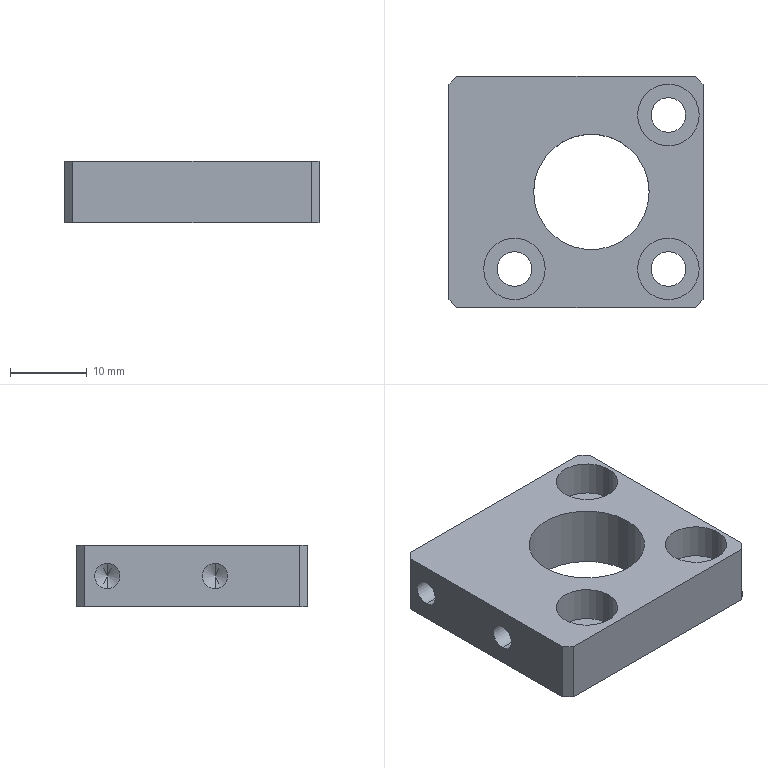Part | STEP file | FBDS-CS-015 | 1 solid | 35 faces | box 33 x 30 x 8 mm | volume 5456 mm3 | cylinder 18 | plane 13 | cone 4 | commonest cylinder face diameters 4.5 x6 8 x6 3.3 x4 15 x2
STEP:
#1=CARTESIAN_POINT('',(-8.4,11.,2.35));
#2=VERTEX_POINT('',#1);
#3=CARTESIAN_POINT('',(-8.4,11.,5.65));
#4=VERTEX_POINT('',#3);
#5=CARTESIAN_POINT('',(-8.4,11.,4.));
#6=DIRECTION('',(-1.,0.,0.));
#7=DIRECTION('',(0.,0.,1.));
#8=AXIS2_PLACEMENT_3D('',#5,#6,#7);
#9=CIRCLE('',#8,1.65);
#10=EDGE_CURVE('',#2,#4,#9,.T.);
#11=ORIENTED_EDGE('',*,*,#10,.F.);
#12=CARTESIAN_POINT('',(-18.5,11.,2.35));
#13=VERTEX_POINT('',#12);
#14=CARTESIAN_POINT('',(-18.5,11.,2.35));
#15=DIRECTION('',(-1.,0.,0.));
#16=VECTOR('',#15,1000.);
#17=LINE('',#14,#16);
#18=EDGE_CURVE('',#2,#13,#17,.T.);
#19=ORIENTED_EDGE('',*,*,#18,.T.);
#20=CARTESIAN_POINT('',(-18.5,11.,5.65));
#21=VERTEX_POINT('',#20);
#22=CARTESIAN_POINT('',(-18.5,11.,4.));
#23=DIRECTION('',(-1.,0.,0.));
#24=DIRECTION('',(0.,0.,1.));
#25=AXIS2_PLACEMENT_3D('',#22,#23,#24);
#26=CIRCLE('',#25,1.65);
#27=EDGE_CURVE('',#13,#21,#26,.T.);
#28=ORIENTED_EDGE('',*,*,#27,.T.);
#29=CARTESIAN_POINT('',(-18.5,11.,5.65));
#30=DIRECTION('',(-1.,0.,0.));
#31=VECTOR('',#30,1000.);
#32=LINE('',#29,#31);
#33=EDGE_CURVE('',#4,#21,#32,.T.);
#34=ORIENTED_EDGE('',*,*,#33,.F.);
#35=EDGE_LOOP('',(#11,#19,#28,#34));
#36=FACE_OUTER_BOUND('',#35,.T.);
#37=CARTESIAN_POINT('',(-18.5,11.,4.));
#38=DIRECTION('',(-1.,0.,0.));
#39=DIRECTION('',(0.,0.,1.));
#40=AXIS2_PLACEMENT_3D('',#37,#38,#39);
#41=CYLINDRICAL_SURFACE('',#40,1.65);
#42=ADVANCED_FACE('',(#36),#41,.F.);
#43=CARTESIAN_POINT('',(-7.409,11.,4.));
#44=VERTEX_POINT('',#43);
#45=CARTESIAN_POINT('',(-8.4,11.,5.65));
#46=DIRECTION('',(-0.515,0.,0.8572));
#47=VECTOR('',#46,1000.);
#48=LINE('',#45,#47);
#49=EDGE_CURVE('',#44,#4,#48,.T.);
#50=ORIENTED_EDGE('',*,*,#49,.F.);
#51=CARTESIAN_POINT('',(-8.4,11.,2.35));
#52=DIRECTION('',(-0.515,0.,-0.8572));
#53=VECTOR('',#52,1000.);
#54=LINE('',#51,#53);
#55=EDGE_CURVE('',#44,#2,#54,.T.);
#56=ORIENTED_EDGE('',*,*,#55,.T.);
#57=ORIENTED_EDGE('',*,*,#10,.T.);
#58=EDGE_LOOP('',(#50,#56,#57));
#59=FACE_OUTER_BOUND('',#58,.T.);
#60=CARTESIAN_POINT('',(-8.4,11.,4.));
#61=DIRECTION('',(-1.,0.,0.));
#62=DIRECTION('',(0.,0.,1.));
#63=AXIS2_PLACEMENT_3D('',#60,#61,#62);
#64=CONICAL_SURFACE('',#63,1.65,1.03);
#65=ADVANCED_FACE('',(#59),#64,.F.);
#66=CARTESIAN_POINT('',(-8.4,-3.,2.35));
#67=VERTEX_POINT('',#66);
#68=CARTESIAN_POINT('',(-8.4,-3.,5.65));
#69=VERTEX_POINT('',#68);
#70=CARTESIAN_POINT('',(-8.4,-3.,4.));
#71=DIRECTION('',(-1.,0.,0.));
#72=DIRECTION('',(0.,0.,1.));
#73=AXIS2_PLACEMENT_3D('',#70,#71,#72);
#74=CIRCLE('',#73,1.65);
#75=EDGE_CURVE('',#67,#69,#74,.T.);
#76=ORIENTED_EDGE('',*,*,#75,.F.);
#77=CARTESIAN_POINT('',(-18.5,-3.,2.35));
#78=VERTEX_POINT('',#77);
#79=CARTESIAN_POINT('',(-18.5,-3.,2.35));
#80=DIRECTION('',(-1.,0.,0.));
#81=VECTOR('',#80,1000.);
#82=LINE('',#79,#81);
#83=EDGE_CURVE('',#67,#78,#82,.T.);
#84=ORIENTED_EDGE('',*,*,#83,.T.);
#85=CARTESIAN_POINT('',(-18.5,-3.,5.65));
#86=VERTEX_POINT('',#85);
#87=CARTESIAN_POINT('',(-18.5,-3.,4.));
#88=DIRECTION('',(-1.,0.,0.));
#89=DIRECTION('',(0.,0.,1.));
#90=AXIS2_PLACEMENT_3D('',#87,#88,#89);
#91=CIRCLE('',#90,1.65);
#92=EDGE_CURVE('',#78,#86,#91,.T.);
#93=ORIENTED_EDGE('',*,*,#92,.T.);
#94=CARTESIAN_POINT('',(-18.5,-3.,5.65));
#95=DIRECTION('',(-1.,0.,0.));
#96=VECTOR('',#95,1000.);
#97=LINE('',#94,#96);
#98=EDGE_CURVE('',#69,#86,#97,.T.);
#99=ORIENTED_EDGE('',*,*,#98,.F.);
#100=EDGE_LOOP('',(#76,#84,#93,#99));
#101=FACE_OUTER_BOUND('',#100,.T.);
#102=CARTESIAN_POINT('',(-18.5,-3.,4.));
#103=DIRECTION('',(-1.,0.,0.));
#104=DIRECTION('',(0.,0.,1.));
#105=AXIS2_PLACEMENT_3D('',#102,#103,#104);
#106=CYLINDRICAL_SURFACE('',#105,1.65);
#107=ADVANCED_FACE('',(#101),#106,.F.);
#108=CARTESIAN_POINT('',(-7.409,-3.,4.));
#109=VERTEX_POINT('',#108);
#110=CARTESIAN_POINT('',(-8.4,-3.,5.65));
#111=DIRECTION('',(-0.515,0.,0.8572));
#112=VECTOR('',#111,1000.);
#113=LINE('',#110,#112);
#114=EDGE_CURVE('',#109,#69,#113,.T.);
#115=ORIENTED_EDGE('',*,*,#114,.F.);
#116=CARTESIAN_POINT('',(-8.4,-3.,2.35));
#117=DIRECTION('',(-0.515,0.,-0.8572));
#118=VECTOR('',#117,1000.);
#119=LINE('',#116,#118);
#120=EDGE_CURVE('',#109,#67,#119,.T.);
#121=ORIENTED_EDGE('',*,*,#120,.T.);
#122=ORIENTED_EDGE('',*,*,#75,.T.);
#123=EDGE_LOOP('',(#115,#121,#122));
#124=FACE_OUTER_BOUND('',#123,.T.);
#125=CARTESIAN_POINT('',(-8.4,-3.,4.));
#126=DIRECTION('',(-1.,0.,0.));
#127=DIRECTION('',(0.,0.,1.));
#128=AXIS2_PLACEMENT_3D('',#125,#126,#127);
#129=CONICAL_SURFACE('',#128,1.65,1.03);
#130=ADVANCED_FACE('',(#124),#129,.F.);
#131=CARTESIAN_POINT('',(-14.,-10.,3.4));
#132=VERTEX_POINT('',#131);
#133=CARTESIAN_POINT('',(-6.,-10.,3.4));
#134=VERTEX_POINT('',#133);
#135=CARTESIAN_POINT('',(-10.,-10.,3.4));
#136=DIRECTION('',(0.,0.,1.));
#137=DIRECTION('',(1.,0.,0.));
#138=AXIS2_PLACEMENT_3D('',#135,#136,#137);
#139=CIRCLE('',#138,4.);
#140=EDGE_CURVE('',#132,#134,#139,.T.);
#141=ORIENTED_EDGE('',*,*,#140,.F.);
#142=CARTESIAN_POINT('',(-14.,-10.,8.));
#143=VERTEX_POINT('',#142);
#144=CARTESIAN_POINT('',(-14.,-10.,8.));
#145=DIRECTION('',(0.,0.,1.));
#146=VECTOR('',#145,1000.);
#147=LINE('',#144,#146);
#148=EDGE_CURVE('',#132,#143,#147,.T.);
#149=ORIENTED_EDGE('',*,*,#148,.T.);
#150=CARTESIAN_POINT('',(-6.,-10.,8.));
#151=VERTEX_POINT('',#150);
#152=CARTESIAN_POINT('',(-10.,-10.,8.));
#153=DIRECTION('',(0.,0.,1.));
#154=DIRECTION('',(1.,0.,0.));
#155=AXIS2_PLACEMENT_3D('',#152,#153,#154);
#156=CIRCLE('',#155,4.);
#157=EDGE_CURVE('',#143,#151,#156,.T.);
#158=ORIENTED_EDGE('',*,*,#157,.T.);
#159=CARTESIAN_POINT('',(-6.,-10.,8.));
#160=DIRECTION('',(0.,0.,1.));
#161=VECTOR('',#160,1000.);
#162=LINE('',#159,#161);
#163=EDGE_CURVE('',#134,#151,#162,.T.);
#164=ORIENTED_EDGE('',*,*,#163,.F.);
#165=EDGE_LOOP('',(#141,#149,#158,#164));
#166=FACE_OUTER_BOUND('',#165,.T.);
#167=CARTESIAN_POINT('',(-10.,-10.,8.));
#168=DIRECTION('',(0.,0.,1.));
#169=DIRECTION('',(1.,0.,0.));
#170=AXIS2_PLACEMENT_3D('',#167,#168,#169);
#171=CYLINDRICAL_SURFACE('',#170,4.);
#172=ADVANCED_FACE('',(#166),#171,.F.);
#173=CARTESIAN_POINT('',(-12.25,-10.,0.));
#174=VERTEX_POINT('',#173);
#175=CARTESIAN_POINT('',(-7.75,-10.,0.));
#176=VERTEX_POINT('',#175);
#177=CARTESIAN_POINT('',(-10.,-10.,0.));
#178=DIRECTION('',(0.,0.,1.));
#179=DIRECTION('',(1.,0.,0.));
#180=AXIS2_PLACEMENT_3D('',#177,#178,#179);
#181=CIRCLE('',#180,2.25);
#182=EDGE_CURVE('',#174,#176,#181,.T.);
#183=ORIENTED_EDGE('',*,*,#182,.F.);
#184=CARTESIAN_POINT('',(-12.25,-10.,3.4));
#185=VERTEX_POINT('',#184);
#186=CARTESIAN_POINT('',(-12.25,-10.,8.));
#187=DIRECTION('',(0.,0.,1.));
#188=VECTOR('',#187,1000.);
#189=LINE('',#186,#188);
#190=EDGE_CURVE('',#174,#185,#189,.T.);
#191=ORIENTED_EDGE('',*,*,#190,.T.);
#192=CARTESIAN_POINT('',(-7.75,-10.,3.4));
#193=VERTEX_POINT('',#192);
#194=CARTESIAN_POINT('',(-10.,-10.,3.4));
#195=DIRECTION('',(0.,0.,1.));
#196=DIRECTION('',(1.,0.,0.));
#197=AXIS2_PLACEMENT_3D('',#194,#195,#196);
#198=CIRCLE('',#197,2.25);
#199=EDGE_CURVE('',#185,#193,#198,.T.);
#200=ORIENTED_EDGE('',*,*,#199,.T.);
#201=CARTESIAN_POINT('',(-7.75,-10.,8.));
#202=DIRECTION('',(0.,0.,1.));
#203=VECTOR('',#202,1000.);
#204=LINE('',#201,#203);
#205=EDGE_CURVE('',#176,#193,#204,.T.);
#206=ORIENTED_EDGE('',*,*,#205,.F.);
#207=EDGE_LOOP('',(#183,#191,#200,#206));
#208=FACE_OUTER_BOUND('',#207,.T.);
#209=CARTESIAN_POINT('',(-10.,-10.,8.));
#210=DIRECTION('',(0.,0.,1.));
#211=DIRECTION('',(1.,0.,0.));
#212=AXIS2_PLACEMENT_3D('',#209,#210,#211);
#213=CYLINDRICAL_SURFACE('',#212,2.25);
#214=ADVANCED_FACE('',(#208),#213,.F.);
#215=CARTESIAN_POINT('',(6.,10.,3.4));
#216=VERTEX_POINT('',#215);
#217=CARTESIAN_POINT('',(14.,10.,3.4));
#218=VERTEX_POINT('',#217);
#219=CARTESIAN_POINT('',(10.,10.,3.4));
#220=DIRECTION('',(0.,0.,1.));
#221=DIRECTION('',(1.,0.,0.));
#222=AXIS2_PLACEMENT_3D('',#219,#220,#221);
#223=CIRCLE('',#222,4.);
#224=EDGE_CURVE('',#216,#218,#223,.T.);
#225=ORIENTED_EDGE('',*,*,#224,.F.);
#226=CARTESIAN_POINT('',(6.,10.,8.));
#227=VERTEX_POINT('',#226);
#228=CARTESIAN_POINT('',(6.,10.,8.));
#229=DIRECTION('',(0.,0.,1.));
#230=VECTOR('',#229,1000.);
#231=LINE('',#228,#230);
#232=EDGE_CURVE('',#216,#227,#231,.T.);
#233=ORIENTED_EDGE('',*,*,#232,.T.);
#234=CARTESIAN_POINT('',(14.,10.,8.));
#235=VERTEX_POINT('',#234);
#236=CARTESIAN_POINT('',(10.,10.,8.));
#237=DIRECTION('',(0.,0.,1.));
#238=DIRECTION('',(1.,0.,0.));
#239=AXIS2_PLACEMENT_3D('',#236,#237,#238);
#240=CIRCLE('',#239,4.);
#241=EDGE_CURVE('',#227,#235,#240,.T.);
#242=ORIENTED_EDGE('',*,*,#241,.T.);
#243=CARTESIAN_POINT('',(14.,10.,8.));
#244=DIRECTION('',(0.,0.,1.));
#245=VECTOR('',#244,1000.);
#246=LINE('',#243,#245);
#247=EDGE_CURVE('',#218,#235,#246,.T.);
#248=ORIENTED_EDGE('',*,*,#247,.F.);
#249=EDGE_LOOP('',(#225,#233,#242,#248));
#250=FACE_OUTER_BOUND('',#249,.T.);
#251=CARTESIAN_POINT('',(10.,10.,8.));
#252=DIRECTION('',(0.,0.,1.));
#253=DIRECTION('',(1.,0.,0.));
#254=AXIS2_PLACEMENT_3D('',#251,#252,#253);
#255=CYLINDRICAL_SURFACE('',#254,4.);
#256=ADVANCED_FACE('',(#250),#255,.F.);
#257=CARTESIAN_POINT('',(7.75,10.,0.));
#258=VERTEX_POINT('',#257);
#259=CARTESIAN_POINT('',(12.25,10.,0.));
#260=VERTEX_POINT('',#259);
#261=CARTESIAN_POINT('',(10.,10.,0.));
#262=DIRECTION('',(0.,0.,1.));
#263=DIRECTION('',(1.,0.,0.));
#264=AXIS2_PLACEMENT_3D('',#261,#262,#263);
#265=CIRCLE('',#264,2.25);
#266=EDGE_CURVE('',#258,#260,#265,.T.);
#267=ORIENTED_EDGE('',*,*,#266,.F.);
#268=CARTESIAN_POINT('',(7.75,10.,3.4));
#269=VERTEX_POINT('',#268);
#270=CARTESIAN_POINT('',(7.75,10.,8.));
#271=DIRECTION('',(0.,0.,1.));
#272=VECTOR('',#271,1000.);
#273=LINE('',#270,#272);
#274=EDGE_CURVE('',#258,#269,#273,.T.);
#275=ORIENTED_EDGE('',*,*,#274,.T.);
#276=CARTESIAN_POINT('',(12.25,10.,3.4));
#277=VERTEX_POINT('',#276);
#278=CARTESIAN_POINT('',(10.,10.,3.4));
#279=DIRECTION('',(0.,0.,1.));
#280=DIRECTION('',(1.,0.,0.));
#281=AXIS2_PLACEMENT_3D('',#278,#279,#280);
#282=CIRCLE('',#281,2.25);
#283=EDGE_CURVE('',#269,#277,#282,.T.);
#284=ORIENTED_EDGE('',*,*,#283,.T.);
#285=CARTESIAN_POINT('',(12.25,10.,8.));
#286=DIRECTION('',(0.,0.,1.));
#287=VECTOR('',#286,1000.);
#288=LINE('',#285,#287);
#289=EDGE_CURVE('',#260,#277,#288,.T.);
#290=ORIENTED_EDGE('',*,*,#289,.F.);
#291=EDGE_LOOP('',(#267,#275,#284,#290));
#292=FACE_OUTER_BOUND('',#291,.T.);
#293=CARTESIAN_POINT('',(10.,10.,8.));
#294=DIRECTION('',(0.,0.,1.));
#295=DIRECTION('',(1.,0.,0.));
#296=AXIS2_PLACEMENT_3D('',#293,#294,#295);
#297=CYLINDRICAL_SURFACE('',#296,2.25);
#298=ADVANCED_FACE('',(#292),#297,.F.);
#299=CARTESIAN_POINT('',(6.,-10.,3.4));
#300=VERTEX_POINT('',#299);
#301=CARTESIAN_POINT('',(14.,-10.,3.4));
#302=VERTEX_POINT('',#301);
#303=CARTESIAN_POINT('',(10.,-10.,3.4));
#304=DIRECTION('',(0.,0.,1.));
#305=DIRECTION('',(1.,0.,0.));
#306=AXIS2_PLACEMENT_3D('',#303,#304,#305);
#307=CIRCLE('',#306,4.);
#308=EDGE_CURVE('',#300,#302,#307,.T.);
#309=ORIENTED_EDGE('',*,*,#308,.F.);
#310=CARTESIAN_POINT('',(6.,-10.,8.));
#311=VERTEX_POINT('',#310);
#312=CARTESIAN_POINT('',(6.,-10.,8.));
#313=DIRECTION('',(0.,0.,1.));
#314=VECTOR('',#313,1000.);
#315=LINE('',#312,#314);
#316=EDGE_CURVE('',#300,#311,#315,.T.);
#317=ORIENTED_EDGE('',*,*,#316,.T.);
#318=CARTESIAN_POINT('',(14.,-10.,8.));
#319=VERTEX_POINT('',#318);
#320=CARTESIAN_POINT('',(10.,-10.,8.));
#321=DIRECTION('',(0.,0.,1.));
#322=DIRECTION('',(1.,0.,0.));
#323=AXIS2_PLACEMENT_3D('',#320,#321,#322);
#324=CIRCLE('',#323,4.);
#325=EDGE_CURVE('',#311,#319,#324,.T.);
#326=ORIENTED_EDGE('',*,*,#325,.T.);
#327=CARTESIAN_POINT('',(14.,-10.,8.));
#328=DIRECTION('',(0.,0.,1.));
#329=VECTOR('',#328,1000.);
#330=LINE('',#327,#329);
#331=EDGE_CURVE('',#302,#319,#330,.T.);
#332=ORIENTED_EDGE('',*,*,#331,.F.);
#333=EDGE_LOOP('',(#309,#317,#326,#332));
#334=FACE_OUTER_BOUND('',#333,.T.);
#335=CARTESIAN_POINT('',(10.,-10.,8.));
#336=DIRECTION('',(0.,0.,1.));
#337=DIRECTION('',(1.,0.,0.));
#338=AXIS2_PLACEMENT_3D('',#335,#336,#337);
#339=CYLINDRICAL_SURFACE('',#338,4.);
#340=ADVANCED_FACE('',(#334),#339,.F.);
#341=CARTESIAN_POINT('',(7.75,-10.,0.));
#342=VERTEX_POINT('',#341);
#343=CARTESIAN_POINT('',(12.25,-10.,0.));
#344=VERTEX_POINT('',#343);
#345=CARTESIAN_POINT('',(10.,-10.,0.));
#346=DIRECTION('',(0.,0.,1.));
#347=DIRECTION('',(1.,0.,0.));
#348=AXIS2_PLACEMENT_3D('',#345,#346,#347);
#349=CIRCLE('',#348,2.25);
#350=EDGE_CURVE('',#342,#344,#349,.T.);
#351=ORIENTED_EDGE('',*,*,#350,.F.);
#352=CARTESIAN_POINT('',(7.75,-10.,3.4));
#353=VERTEX_POINT('',#352);
#354=CARTESIAN_POINT('',(7.75,-10.,8.));
#355=DIRECTION('',(0.,0.,1.));
#356=VECTOR('',#355,1000.);
#357=LINE('',#354,#356);
#358=EDGE_CURVE('',#342,#353,#357,.T.);
#359=ORIENTED_EDGE('',*,*,#358,.T.);
#360=CARTESIAN_POINT('',(12.25,-10.,3.4));
#361=VERTEX_POINT('',#360);
#362=CARTESIAN_POINT('',(10.,-10.,3.4));
#363=DIRECTION('',(0.,0.,1.));
#364=DIRECTION('',(1.,0.,0.));
#365=AXIS2_PLACEMENT_3D('',#362,#363,#364);
#366=CIRCLE('',#365,2.25);
#367=EDGE_CURVE('',#353,#361,#366,.T.);
#368=ORIENTED_EDGE('',*,*,#367,.T.);
#369=CARTESIAN_POINT('',(12.25,-10.,8.));
#370=DIRECTION('',(0.,0.,1.));
#371=VECTOR('',#370,1000.);
#372=LINE('',#369,#371);
#373=EDGE_CURVE('',#344,#361,#372,.T.);
#374=ORIENTED_EDGE('',*,*,#373,.F.);
#375=EDGE_LOOP('',(#351,#359,#368,#374));
#376=FACE_OUTER_BOUND('',#375,.T.);
#377=CARTESIAN_POINT('',(10.,-10.,8.));
#378=DIRECTION('',(0.,0.,1.));
#379=DIRECTION('',(1.,0.,0.));
#380=AXIS2_PLACEMENT_3D('',#377,#378,#379);
#381=CYLINDRICAL_SURFACE('',#380,2.25);
#382=ADVANCED_FACE('',(#376),#381,.F.);
#383=CARTESIAN_POINT('',(7.5,0.,0.));
#384=VERTEX_POINT('',#383);
#385=CARTESIAN_POINT('',(-7.5,0.,0.));
#386=VERTEX_POINT('',#385);
#387=CARTESIAN_POINT('',(0.,0.,0.));
#388=DIRECTION('',(0.,0.,-1.));
#389=DIRECTION('',(-1.,0.,0.));
#390=AXIS2_PLACEMENT_3D('',#387,#388,#389);
#391=CIRCLE('',#390,7.5);
#392=EDGE_CURVE('',#384,#386,#391,.T.);
#393=ORIENTED_EDGE('',*,*,#392,.T.);
#394=CARTESIAN_POINT('',(-7.5,0.,8.));
#395=VERTEX_POINT('',#394);
#396=CARTESIAN_POINT('',(-7.5,0.,-7.));
#397=DIRECTION('',(0.,0.,1.));
#398=VECTOR('',#397,1000.);
#399=LINE('',#396,#398);
#400=EDGE_CURVE('',#386,#395,#399,.T.);
#401=ORIENTED_EDGE('',*,*,#400,.T.);
#402=CARTESIAN_POINT('',(7.5,0.,8.));
#403=VERTEX_POINT('',#402);
#404=CARTESIAN_POINT('',(0.,0.,8.));
#405=DIRECTION('',(0.,0.,1.));
#406=DIRECTION('',(1.,0.,0.));
#407=AXIS2_PLACEMENT_3D('',#404,#405,#406);
#408=CIRCLE('',#407,7.5);
#409=EDGE_CURVE('',#395,#403,#408,.T.);
#410=ORIENTED_EDGE('',*,*,#409,.T.);
#411=CARTESIAN_POINT('',(7.5,0.,-7.));
#412=DIRECTION('',(0.,0.,1.));
#413=VECTOR('',#412,1000.);
#414=LINE('',#411,#413);
#415=EDGE_CURVE('',#384,#403,#414,.T.);
#416=ORIENTED_EDGE('',*,*,#415,.F.);
#417=EDGE_LOOP('',(#393,#401,#410,#416));
#418=FACE_OUTER_BOUND('',#417,.T.);
#419=CARTESIAN_POINT('',(0.,0.,-7.));
#420=DIRECTION('',(0.,0.,1.));
#421=DIRECTION('',(1.,0.,0.));
#422=AXIS2_PLACEMENT_3D('',#419,#420,#421);
#423=CYLINDRICAL_SURFACE('',#422,7.5);
#424=ADVANCED_FACE('',(#418),#423,.F.);
#425=CARTESIAN_POINT('',(14.5,-14.,8.));
#426=VERTEX_POINT('',#425);
#427=CARTESIAN_POINT('',(14.5,14.,8.));
#428=VERTEX_POINT('',#427);
#429=CARTESIAN_POINT('',(14.5,-15.,8.));
#430=DIRECTION('',(0.,1.,0.));
#431=VECTOR('',#430,1000.);
#432=LINE('',#429,#431);
#433=EDGE_CURVE('',#426,#428,#432,.T.);
#434=ORIENTED_EDGE('',*,*,#433,.F.);
#435=CARTESIAN_POINT('',(14.5,-14.,0.));
#436=VERTEX_POINT('',#435);
#437=CARTESIAN_POINT('',(14.5,-14.,8.));
#438=DIRECTION('',(0.,0.,-1.));
#439=VECTOR('',#438,1000.);
#440=LINE('',#437,#439);
#441=EDGE_CURVE('',#426,#436,#440,.T.);
#442=ORIENTED_EDGE('',*,*,#441,.T.);
#443=CARTESIAN_POINT('',(14.5,14.,0.));
#444=VERTEX_POINT('',#443);
#445=CARTESIAN_POINT('',(14.5,-15.,0.));
#446=DIRECTION('',(0.,1.,0.));
#447=VECTOR('',#446,1000.);
#448=LINE('',#445,#447);
#449=EDGE_CURVE('',#436,#444,#448,.T.);
#450=ORIENTED_EDGE('',*,*,#449,.T.);
#451=CARTESIAN_POINT('',(14.5,14.,8.));
#452=DIRECTION('',(0.,0.,1.));
#453=VECTOR('',#452,1000.);
#454=LINE('',#451,#453);
#455=EDGE_CURVE('',#444,#428,#454,.T.);
#456=ORIENTED_EDGE('',*,*,#455,.T.);
#457=EDGE_LOOP('',(#434,#442,#450,#456));
#458=FACE_OUTER_BOUND('',#457,.T.);
#459=CARTESIAN_POINT('',(14.5,-15.,8.));
#460=DIRECTION('',(-1.,0.,0.));
#461=DIRECTION('',(0.,0.,1.));
#462=AXIS2_PLACEMENT_3D('',#459,#460,#461);
#463=PLANE('',#462);
#464=ADVANCED_FACE('',(#458),#463,.F.);
#465=CARTESIAN_POINT('',(13.5,15.,0.));
#466=VERTEX_POINT('',#465);
#467=CARTESIAN_POINT('',(-17.5,15.,0.));
#468=VERTEX_POINT('',#467);
#469=CARTESIAN_POINT('',(-14.5,15.,0.));
#470=DIRECTION('',(-1.,0.,0.));
#471=VECTOR('',#470,1000.);
#472=LINE('',#469,#471);
#473=EDGE_CURVE('',#466,#468,#472,.T.);
#474=ORIENTED_EDGE('',*,*,#473,.T.);
#475=CARTESIAN_POINT('',(-17.5,15.,8.));
#476=VERTEX_POINT('',#475);
#477=CARTESIAN_POINT('',(-17.5,15.,8.));
#478=DIRECTION('',(0.,0.,1.));
#479=VECTOR('',#478,1000.);
#480=LINE('',#477,#479);
#481=EDGE_CURVE('',#468,#476,#480,.T.);
#482=ORIENTED_EDGE('',*,*,#481,.T.);
#483=CARTESIAN_POINT('',(13.5,15.,8.));
#484=VERTEX_POINT('',#483);
#485=CARTESIAN_POINT('',(-14.5,15.,8.));
#486=DIRECTION('',(-1.,0.,0.));
#487=VECTOR('',#486,1000.);
#488=LINE('',#485,#487);
#489=EDGE_CURVE('',#484,#476,#488,.T.);
#490=ORIENTED_EDGE('',*,*,#489,.F.);
#491=CARTESIAN_POINT('',(13.5,15.,8.));
#492=DIRECTION('',(0.,0.,-1.));
#493=VECTOR('',#492,1000.);
#494=LINE('',#491,#493);
#495=EDGE_CURVE('',#484,#466,#494,.T.);
#496=ORIENTED_EDGE('',*,*,#495,.T.);
#497=EDGE_LOOP('',(#474,#482,#490,#496));
#498=FACE_OUTER_BOUND('',#497,.T.);
#499=CARTESIAN_POINT('',(-14.5,15.,8.));
#500=DIRECTION('',(0.,-1.,0.));
#501=DIRECTION('',(0.,0.,-1.));
#502=AXIS2_PLACEMENT_3D('',#499,#500,#501);
#503=PLANE('',#502);
#504=ADVANCED_FACE('',(#498),#503,.F.);
#505=CARTESIAN_POINT('',(-17.5,-15.,8.));
#506=VERTEX_POINT('',#505);
#507=CARTESIAN_POINT('',(13.5,-15.,8.));
#508=VERTEX_POINT('',#507);
#509=CARTESIAN_POINT('',(-14.5,-15.,8.));
#510=DIRECTION('',(1.,0.,0.));
#511=VECTOR('',#510,1000.);
#512=LINE('',#509,#511);
#513=EDGE_CURVE('',#506,#508,#512,.T.);
#514=ORIENTED_EDGE('',*,*,#513,.F.);
#515=CARTESIAN_POINT('',(-17.5,-15.,0.));
#516=VERTEX_POINT('',#515);
#517=CARTESIAN_POINT('',(-17.5,-15.,0.));
#518=DIRECTION('',(0.,0.,-1.));
#519=VECTOR('',#518,1000.);
#520=LINE('',#517,#519);
#521=EDGE_CURVE('',#506,#516,#520,.T.);
#522=ORIENTED_EDGE('',*,*,#521,.T.);
#523=CARTESIAN_POINT('',(13.5,-15.,0.));
#524=VERTEX_POINT('',#523);
#525=CARTESIAN_POINT('',(-14.5,-15.,0.));
#526=DIRECTION('',(1.,0.,0.));
#527=VECTOR('',#526,1000.);
#528=LINE('',#525,#527);
#529=EDGE_CURVE('',#516,#524,#528,.T.);
#530=ORIENTED_EDGE('',*,*,#529,.T.);
#531=CARTESIAN_POINT('',(13.5,-15.,8.));
#532=DIRECTION('',(0.,0.,1.));
#533=VECTOR('',#532,1000.);
#534=LINE('',#531,#533);
#535=EDGE_CURVE('',#524,#508,#534,.T.);
#536=ORIENTED_EDGE('',*,*,#535,.T.);
#537=EDGE_LOOP('',(#514,#522,#530,#536));
#538=FACE_OUTER_BOUND('',#537,.T.);
#539=CARTESIAN_POINT('',(-14.5,-15.,8.));
#540=DIRECTION('',(0.,1.,0.));
#541=DIRECTION('',(0.,0.,1.));
#542=AXIS2_PLACEMENT_3D('',#539,#540,#541);
#543=PLANE('',#542);
#544=ADVANCED_FACE('',(#538),#543,.F.);
#545=CARTESIAN_POINT('',(-10.,-10.,8.));
#546=DIRECTION('',(0.,0.,1.));
#547=DIRECTION('',(1.,0.,0.));
#548=AXIS2_PLACEMENT_3D('',#545,#546,#547);
#549=CIRCLE('',#548,4.);
#550=EDGE_CURVE('',#151,#143,#549,.T.);
#551=ORIENTED_EDGE('',*,*,#550,.F.);
#552=ORIENTED_EDGE('',*,*,#157,.F.);
#553=EDGE_LOOP('',(#551,#552));
#554=FACE_BOUND('',#553,.T.);
#555=CARTESIAN_POINT('',(10.,10.,8.));
#556=DIRECTION('',(0.,0.,1.));
#557=DIRECTION('',(1.,0.,0.));
#558=AXIS2_PLACEMENT_3D('',#555,#556,#557);
#559=CIRCLE('',#558,4.);
#560=EDGE_CURVE('',#235,#227,#559,.T.);
#561=ORIENTED_EDGE('',*,*,#560,.F.);
#562=ORIENTED_EDGE('',*,*,#241,.F.);
#563=EDGE_LOOP('',(#561,#562));
#564=FACE_BOUND('',#563,.T.);
#565=CARTESIAN_POINT('',(10.,-10.,8.));
#566=DIRECTION('',(0.,0.,1.));
#567=DIRECTION('',(1.,0.,0.));
#568=AXIS2_PLACEMENT_3D('',#565,#566,#567);
#569=CIRCLE('',#568,4.);
#570=EDGE_CURVE('',#319,#311,#569,.T.);
#571=ORIENTED_EDGE('',*,*,#570,.F.);
#572=ORIENTED_EDGE('',*,*,#325,.F.);
#573=EDGE_LOOP('',(#571,#572));
#574=FACE_BOUND('',#573,.T.);
#575=CARTESIAN_POINT('',(0.,0.,8.));
#576=DIRECTION('',(0.,0.,1.));
#577=DIRECTION('',(1.,0.,0.));
#578=AXIS2_PLACEMENT_3D('',#575,#576,#577);
#579=CIRCLE('',#578,7.5);
#580=EDGE_CURVE('',#403,#395,#579,.T.);
#581=ORIENTED_EDGE('',*,*,#580,.F.);
#582=ORIENTED_EDGE('',*,*,#409,.F.);
#583=EDGE_LOOP('',(#581,#582));
#584=FACE_BOUND('',#583,.T.);
#585=ORIENTED_EDGE('',*,*,#489,.T.);
#586=CARTESIAN_POINT('',(-18.5,14.,8.));
#587=VERTEX_POINT('',#586);
#588=CARTESIAN_POINT('',(-18.5,14.,8.));
#589=DIRECTION('',(-0.7071,-0.7071,0.));
#590=VECTOR('',#589,1000.);
#591=LINE('',#588,#590);
#592=EDGE_CURVE('',#476,#587,#591,.T.);
#593=ORIENTED_EDGE('',*,*,#592,.T.);
#594=CARTESIAN_POINT('',(-18.5,-14.,8.));
#595=VERTEX_POINT('',#594);
#596=CARTESIAN_POINT('',(-18.5,-15.,8.));
#597=DIRECTION('',(0.,1.,0.));
#598=VECTOR('',#597,1000.);
#599=LINE('',#596,#598);
#600=EDGE_CURVE('',#595,#587,#599,.T.);
#601=ORIENTED_EDGE('',*,*,#600,.F.);
#602=CARTESIAN_POINT('',(-18.5,-14.,8.));
#603=DIRECTION('',(0.7071,-0.7071,0.));
#604=VECTOR('',#603,1000.);
#605=LINE('',#602,#604);
#606=EDGE_CURVE('',#595,#506,#605,.T.);
#607=ORIENTED_EDGE('',*,*,#606,.T.);
#608=ORIENTED_EDGE('',*,*,#513,.T.);
#609=CARTESIAN_POINT('',(14.5,-14.,8.));
#610=DIRECTION('',(0.7071,0.7071,0.));
#611=VECTOR('',#610,1000.);
#612=LINE('',#609,#611);
#613=EDGE_CURVE('',#508,#426,#612,.T.);
#614=ORIENTED_EDGE('',*,*,#613,.T.);
#615=ORIENTED_EDGE('',*,*,#433,.T.);
#616=CARTESIAN_POINT('',(13.5,15.,8.));
#617=DIRECTION('',(-0.7071,0.7071,0.));
#618=VECTOR('',#617,1000.);
#619=LINE('',#616,#618);
#620=EDGE_CURVE('',#428,#484,#619,.T.);
#621=ORIENTED_EDGE('',*,*,#620,.T.);
#622=EDGE_LOOP('',(#585,#593,#601,#607,#608,#614,#615,#621));
#623=FACE_OUTER_BOUND('',#622,.T.);
#624=CARTESIAN_POINT('',(0.,0.,8.));
#625=DIRECTION('',(0.,0.,-1.));
#626=DIRECTION('',(-1.,0.,0.));
#627=AXIS2_PLACEMENT_3D('',#624,#625,#626);
#628=PLANE('',#627);
#629=ADVANCED_FACE('',(#554,#564,#574,#584,#623),#628,.F.);
#630=CARTESIAN_POINT('',(-10.,-10.,0.));
#631=DIRECTION('',(0.,0.,1.));
#632=DIRECTION('',(1.,0.,0.));
#633=AXIS2_PLACEMENT_3D('',#630,#631,#632);
#634=CIRCLE('',#633,2.25);
#635=EDGE_CURVE('',#176,#174,#634,.T.);
#636=ORIENTED_EDGE('',*,*,#635,.T.);
#637=ORIENTED_EDGE('',*,*,#182,.T.);
#638=EDGE_LOOP('',(#636,#637));
#639=FACE_BOUND('',#638,.T.);
#640=CARTESIAN_POINT('',(10.,10.,0.));
#641=DIRECTION('',(0.,0.,1.));
#642=DIRECTION('',(1.,0.,0.));
#643=AXIS2_PLACEMENT_3D('',#640,#641,#642);
#644=CIRCLE('',#643,2.25);
#645=EDGE_CURVE('',#260,#258,#644,.T.);
#646=ORIENTED_EDGE('',*,*,#645,.T.);
#647=ORIENTED_EDGE('',*,*,#266,.T.);
#648=EDGE_LOOP('',(#646,#647));
#649=FACE_BOUND('',#648,.T.);
#650=CARTESIAN_POINT('',(10.,-10.,0.));
#651=DIRECTION('',(0.,0.,1.));
#652=DIRECTION('',(1.,0.,0.));
#653=AXIS2_PLACEMENT_3D('',#650,#651,#652);
#654=CIRCLE('',#653,2.25);
#655=EDGE_CURVE('',#344,#342,#654,.T.);
#656=ORIENTED_EDGE('',*,*,#655,.T.);
#657=ORIENTED_EDGE('',*,*,#350,.T.);
#658=EDGE_LOOP('',(#656,#657));
#659=FACE_BOUND('',#658,.T.);
#660=ORIENTED_EDGE('',*,*,#392,.F.);
#661=CARTESIAN_POINT('',(0.,0.,0.));
#662=DIRECTION('',(0.,0.,-1.));
#663=DIRECTION('',(-1.,0.,0.));
#664=AXIS2_PLACEMENT_3D('',#661,#662,#663);
#665=CIRCLE('',#664,7.5);
#666=EDGE_CURVE('',#386,#384,#665,.T.);
#667=ORIENTED_EDGE('',*,*,#666,.F.);
#668=EDGE_LOOP('',(#660,#667));
#669=FACE_BOUND('',#668,.T.);
#670=CARTESIAN_POINT('',(-18.5,14.,0.));
#671=VERTEX_POINT('',#670);
#672=CARTESIAN_POINT('',(-18.5,-14.,0.));
#673=VERTEX_POINT('',#672);
#674=CARTESIAN_POINT('',(-18.5,15.,0.));
#675=DIRECTION('',(0.,-1.,0.));
#676=VECTOR('',#675,1000.);
#677=LINE('',#674,#676);
#678=EDGE_CURVE('',#671,#673,#677,.T.);
#679=ORIENTED_EDGE('',*,*,#678,.F.);
#680=CARTESIAN_POINT('',(-16.25,16.25,0.));
#681=DIRECTION('',(0.7071,0.7071,0.));
#682=VECTOR('',#681,1000.);
#683=LINE('',#680,#682);
#684=EDGE_CURVE('',#671,#468,#683,.T.);
#685=ORIENTED_EDGE('',*,*,#684,.T.);
#686=ORIENTED_EDGE('',*,*,#473,.F.);
#687=CARTESIAN_POINT('',(14.25,14.25,0.));
#688=DIRECTION('',(0.7071,-0.7071,0.));
#689=VECTOR('',#688,1000.);
#690=LINE('',#687,#689);
#691=EDGE_CURVE('',#466,#444,#690,.T.);
#692=ORIENTED_EDGE('',*,*,#691,.T.);
#693=ORIENTED_EDGE('',*,*,#449,.F.);
#694=CARTESIAN_POINT('',(14.25,-14.25,0.));
#695=DIRECTION('',(-0.7071,-0.7071,0.));
#696=VECTOR('',#695,1000.);
#697=LINE('',#694,#696);
#698=EDGE_CURVE('',#436,#524,#697,.T.);
#699=ORIENTED_EDGE('',*,*,#698,.T.);
#700=ORIENTED_EDGE('',*,*,#529,.F.);
#701=CARTESIAN_POINT('',(-16.25,-16.25,0.));
#702=DIRECTION('',(-0.7071,0.7071,0.));
#703=VECTOR('',#702,1000.);
#704=LINE('',#701,#703);
#705=EDGE_CURVE('',#516,#673,#704,.T.);
#706=ORIENTED_EDGE('',*,*,#705,.T.);
#707=EDGE_LOOP('',(#679,#685,#686,#692,#693,#699,#700,#706));
#708=FACE_OUTER_BOUND('',#707,.T.);
#709=CARTESIAN_POINT('',(0.,0.,0.));
#710=DIRECTION('',(0.,0.,-1.));
#711=DIRECTION('',(-1.,0.,0.));
#712=AXIS2_PLACEMENT_3D('',#709,#710,#711);
#713=PLANE('',#712);
#714=ADVANCED_FACE('',(#639,#649,#659,#669,#708),#713,.T.);
#715=ORIENTED_EDGE('',*,*,#400,.F.);
#716=ORIENTED_EDGE('',*,*,#666,.T.);
#717=ORIENTED_EDGE('',*,*,#415,.T.);
#718=ORIENTED_EDGE('',*,*,#580,.T.);
#719=EDGE_LOOP('',(#715,#716,#717,#718));
#720=FACE_OUTER_BOUND('',#719,.T.);
#721=CARTESIAN_POINT('',(0.,0.,-7.));
#722=DIRECTION('',(0.,0.,1.));
#723=DIRECTION('',(1.,0.,0.));
#724=AXIS2_PLACEMENT_3D('',#721,#722,#723);
#725=CYLINDRICAL_SURFACE('',#724,7.5);
#726=ADVANCED_FACE('',(#720),#725,.F.);
#727=ORIENTED_EDGE('',*,*,#358,.F.);
#728=ORIENTED_EDGE('',*,*,#655,.F.);
#729=ORIENTED_EDGE('',*,*,#373,.T.);
#730=CARTESIAN_POINT('',(10.,-10.,3.4));
#731=DIRECTION('',(0.,0.,1.));
#732=DIRECTION('',(1.,0.,0.));
#733=AXIS2_PLACEMENT_3D('',#730,#731,#732);
#734=CIRCLE('',#733,2.25);
#735=EDGE_CURVE('',#361,#353,#734,.T.);
#736=ORIENTED_EDGE('',*,*,#735,.T.);
#737=EDGE_LOOP('',(#727,#728,#729,#736));
#738=FACE_OUTER_BOUND('',#737,.T.);
#739=CARTESIAN_POINT('',(10.,-10.,8.));
#740=DIRECTION('',(0.,0.,1.));
#741=DIRECTION('',(1.,0.,0.));
#742=AXIS2_PLACEMENT_3D('',#739,#740,#741);
#743=CYLINDRICAL_SURFACE('',#742,2.25);
#744=ADVANCED_FACE('',(#738),#743,.F.);
#745=ORIENTED_EDGE('',*,*,#735,.F.);
#746=ORIENTED_EDGE('',*,*,#367,.F.);
#747=EDGE_LOOP('',(#745,#746));
#748=FACE_BOUND('',#747,.T.);
#749=CARTESIAN_POINT('',(10.,-10.,3.4));
#750=DIRECTION('',(0.,0.,1.));
#751=DIRECTION('',(1.,0.,0.));
#752=AXIS2_PLACEMENT_3D('',#749,#750,#751);
#753=CIRCLE('',#752,4.);
#754=EDGE_CURVE('',#302,#300,#753,.T.);
#755=ORIENTED_EDGE('',*,*,#754,.T.);
#756=ORIENTED_EDGE('',*,*,#308,.T.);
#757=EDGE_LOOP('',(#755,#756));
#758=FACE_OUTER_BOUND('',#757,.T.);
#759=CARTESIAN_POINT('',(12.25,-10.,3.4));
#760=DIRECTION('',(0.,0.,-1.));
#761=DIRECTION('',(-1.,0.,0.));
#762=AXIS2_PLACEMENT_3D('',#759,#760,#761);
#763=PLANE('',#762);
#764=ADVANCED_FACE('',(#748,#758),#763,.F.);
#765=ORIENTED_EDGE('',*,*,#316,.F.);
#766=ORIENTED_EDGE('',*,*,#754,.F.);
#767=ORIENTED_EDGE('',*,*,#331,.T.);
#768=ORIENTED_EDGE('',*,*,#570,.T.);
#769=EDGE_LOOP('',(#765,#766,#767,#768));
#770=FACE_OUTER_BOUND('',#769,.T.);
#771=CARTESIAN_POINT('',(10.,-10.,8.));
#772=DIRECTION('',(0.,0.,1.));
#773=DIRECTION('',(1.,0.,0.));
#774=AXIS2_PLACEMENT_3D('',#771,#772,#773);
#775=CYLINDRICAL_SURFACE('',#774,4.);
#776=ADVANCED_FACE('',(#770),#775,.F.);
#777=ORIENTED_EDGE('',*,*,#274,.F.);
#778=ORIENTED_EDGE('',*,*,#645,.F.);
#779=ORIENTED_EDGE('',*,*,#289,.T.);
#780=CARTESIAN_POINT('',(10.,10.,3.4));
#781=DIRECTION('',(0.,0.,1.));
#782=DIRECTION('',(1.,0.,0.));
#783=AXIS2_PLACEMENT_3D('',#780,#781,#782);
#784=CIRCLE('',#783,2.25);
#785=EDGE_CURVE('',#277,#269,#784,.T.);
#786=ORIENTED_EDGE('',*,*,#785,.T.);
#787=EDGE_LOOP('',(#777,#778,#779,#786));
#788=FACE_OUTER_BOUND('',#787,.T.);
#789=CARTESIAN_POINT('',(10.,10.,8.));
#790=DIRECTION('',(0.,0.,1.));
#791=DIRECTION('',(1.,0.,0.));
#792=AXIS2_PLACEMENT_3D('',#789,#790,#791);
#793=CYLINDRICAL_SURFACE('',#792,2.25);
#794=ADVANCED_FACE('',(#788),#793,.F.);
#795=ORIENTED_EDGE('',*,*,#785,.F.);
#796=ORIENTED_EDGE('',*,*,#283,.F.);
#797=EDGE_LOOP('',(#795,#796));
#798=FACE_BOUND('',#797,.T.);
#799=CARTESIAN_POINT('',(10.,10.,3.4));
#800=DIRECTION('',(0.,0.,1.));
#801=DIRECTION('',(1.,0.,0.));
#802=AXIS2_PLACEMENT_3D('',#799,#800,#801);
#803=CIRCLE('',#802,4.);
#804=EDGE_CURVE('',#218,#216,#803,.T.);
#805=ORIENTED_EDGE('',*,*,#804,.T.);
#806=ORIENTED_EDGE('',*,*,#224,.T.);
#807=EDGE_LOOP('',(#805,#806));
#808=FACE_OUTER_BOUND('',#807,.T.);
#809=CARTESIAN_POINT('',(12.25,10.,3.4));
#810=DIRECTION('',(0.,0.,-1.));
#811=DIRECTION('',(-1.,0.,0.));
#812=AXIS2_PLACEMENT_3D('',#809,#810,#811);
#813=PLANE('',#812);
#814=ADVANCED_FACE('',(#798,#808),#813,.F.);
#815=ORIENTED_EDGE('',*,*,#232,.F.);
#816=ORIENTED_EDGE('',*,*,#804,.F.);
#817=ORIENTED_EDGE('',*,*,#247,.T.);
#818=ORIENTED_EDGE('',*,*,#560,.T.);
#819=EDGE_LOOP('',(#815,#816,#817,#818));
#820=FACE_OUTER_BOUND('',#819,.T.);
#821=CARTESIAN_POINT('',(10.,10.,8.));
#822=DIRECTION('',(0.,0.,1.));
#823=DIRECTION('',(1.,0.,0.));
#824=AXIS2_PLACEMENT_3D('',#821,#822,#823);
#825=CYLINDRICAL_SURFACE('',#824,4.);
#826=ADVANCED_FACE('',(#820),#825,.F.);
#827=ORIENTED_EDGE('',*,*,#190,.F.);
#828=ORIENTED_EDGE('',*,*,#635,.F.);
#829=ORIENTED_EDGE('',*,*,#205,.T.);
#830=CARTESIAN_POINT('',(-10.,-10.,3.4));
#831=DIRECTION('',(0.,0.,1.));
#832=DIRECTION('',(1.,0.,0.));
#833=AXIS2_PLACEMENT_3D('',#830,#831,#832);
#834=CIRCLE('',#833,2.25);
#835=EDGE_CURVE('',#193,#185,#834,.T.);
#836=ORIENTED_EDGE('',*,*,#835,.T.);
#837=EDGE_LOOP('',(#827,#828,#829,#836));
#838=FACE_OUTER_BOUND('',#837,.T.);
#839=CARTESIAN_POINT('',(-10.,-10.,8.));
#840=DIRECTION('',(0.,0.,1.));
#841=DIRECTION('',(1.,0.,0.));
#842=AXIS2_PLACEMENT_3D('',#839,#840,#841);
#843=CYLINDRICAL_SURFACE('',#842,2.25);
#844=ADVANCED_FACE('',(#838),#843,.F.);
#845=ORIENTED_EDGE('',*,*,#835,.F.);
#846=ORIENTED_EDGE('',*,*,#199,.F.);
#847=EDGE_LOOP('',(#845,#846));
#848=FACE_BOUND('',#847,.T.);
#849=CARTESIAN_POINT('',(-10.,-10.,3.4));
#850=DIRECTION('',(0.,0.,1.));
#851=DIRECTION('',(1.,0.,0.));
#852=AXIS2_PLACEMENT_3D('',#849,#850,#851);
#853=CIRCLE('',#852,4.);
#854=EDGE_CURVE('',#134,#132,#853,.T.);
#855=ORIENTED_EDGE('',*,*,#854,.T.);
#856=ORIENTED_EDGE('',*,*,#140,.T.);
#857=EDGE_LOOP('',(#855,#856));
#858=FACE_OUTER_BOUND('',#857,.T.);
#859=CARTESIAN_POINT('',(-7.75,-10.,3.4));
#860=DIRECTION('',(0.,0.,-1.));
#861=DIRECTION('',(-1.,0.,0.));
#862=AXIS2_PLACEMENT_3D('',#859,#860,#861);
#863=PLANE('',#862);
#864=ADVANCED_FACE('',(#848,#858),#863,.F.);
#865=ORIENTED_EDGE('',*,*,#148,.F.);
#866=ORIENTED_EDGE('',*,*,#854,.F.);
#867=ORIENTED_EDGE('',*,*,#163,.T.);
#868=ORIENTED_EDGE('',*,*,#550,.T.);
#869=EDGE_LOOP('',(#865,#866,#867,#868));
#870=FACE_OUTER_BOUND('',#869,.T.);
#871=CARTESIAN_POINT('',(-10.,-10.,8.));
#872=DIRECTION('',(0.,0.,1.));
#873=DIRECTION('',(1.,0.,0.));
#874=AXIS2_PLACEMENT_3D('',#871,#872,#873);
#875=CYLINDRICAL_SURFACE('',#874,4.);
#876=ADVANCED_FACE('',(#870),#875,.F.);
#877=CARTESIAN_POINT('',(-18.5,11.,4.));
#878=DIRECTION('',(-1.,0.,0.));
#879=DIRECTION('',(0.,0.,1.));
#880=AXIS2_PLACEMENT_3D('',#877,#878,#879);
#881=CIRCLE('',#880,1.65);
#882=EDGE_CURVE('',#21,#13,#881,.T.);
#883=ORIENTED_EDGE('',*,*,#882,.F.);
#884=ORIENTED_EDGE('',*,*,#27,.F.);
#885=EDGE_LOOP('',(#883,#884));
#886=FACE_BOUND('',#885,.T.);
#887=CARTESIAN_POINT('',(-18.5,-3.,4.));
#888=DIRECTION('',(-1.,0.,0.));
#889=DIRECTION('',(0.,0.,1.));
#890=AXIS2_PLACEMENT_3D('',#887,#888,#889);
#891=CIRCLE('',#890,1.65);
#892=EDGE_CURVE('',#86,#78,#891,.T.);
#893=ORIENTED_EDGE('',*,*,#892,.F.);
#894=ORIENTED_EDGE('',*,*,#92,.F.);
#895=EDGE_LOOP('',(#893,#894));
#896=FACE_BOUND('',#895,.T.);
#897=ORIENTED_EDGE('',*,*,#600,.T.);
#898=CARTESIAN_POINT('',(-18.5,14.,0.));
#899=DIRECTION('',(0.,0.,-1.));
#900=VECTOR('',#899,1000.);
#901=LINE('',#898,#900);
#902=EDGE_CURVE('',#587,#671,#901,.T.);
#903=ORIENTED_EDGE('',*,*,#902,.T.);
#904=ORIENTED_EDGE('',*,*,#678,.T.);
#905=CARTESIAN_POINT('',(-18.5,-14.,8.));
#906=DIRECTION('',(0.,0.,1.));
#907=VECTOR('',#906,1000.);
#908=LINE('',#905,#907);
#909=EDGE_CURVE('',#673,#595,#908,.T.);
#910=ORIENTED_EDGE('',*,*,#909,.T.);
#911=EDGE_LOOP('',(#897,#903,#904,#910));
#912=FACE_OUTER_BOUND('',#911,.T.);
#913=CARTESIAN_POINT('',(-18.5,0.,0.));
#914=DIRECTION('',(-1.,0.,0.));
#915=DIRECTION('',(0.,0.,1.));
#916=AXIS2_PLACEMENT_3D('',#913,#914,#915);
#917=PLANE('',#916);
#918=ADVANCED_FACE('',(#886,#896,#912),#917,.T.);
#919=ORIENTED_EDGE('',*,*,#120,.F.);
#920=ORIENTED_EDGE('',*,*,#114,.T.);
#921=CARTESIAN_POINT('',(-8.4,-3.,4.));
#922=DIRECTION('',(-1.,0.,0.));
#923=DIRECTION('',(0.,0.,1.));
#924=AXIS2_PLACEMENT_3D('',#921,#922,#923);
#925=CIRCLE('',#924,1.65);
#926=EDGE_CURVE('',#69,#67,#925,.T.);
#927=ORIENTED_EDGE('',*,*,#926,.T.);
#928=EDGE_LOOP('',(#919,#920,#927));
#929=FACE_OUTER_BOUND('',#928,.T.);
#930=CARTESIAN_POINT('',(-8.4,-3.,4.));
#931=DIRECTION('',(-1.,0.,0.));
#932=DIRECTION('',(0.,0.,1.));
#933=AXIS2_PLACEMENT_3D('',#930,#931,#932);
#934=CONICAL_SURFACE('',#933,1.65,1.03);
#935=ADVANCED_FACE('',(#929),#934,.F.);
#936=ORIENTED_EDGE('',*,*,#83,.F.);
#937=ORIENTED_EDGE('',*,*,#926,.F.);
#938=ORIENTED_EDGE('',*,*,#98,.T.);
#939=ORIENTED_EDGE('',*,*,#892,.T.);
#940=EDGE_LOOP('',(#936,#937,#938,#939));
#941=FACE_OUTER_BOUND('',#940,.T.);
#942=CARTESIAN_POINT('',(-18.5,-3.,4.));
#943=DIRECTION('',(-1.,0.,0.));
#944=DIRECTION('',(0.,0.,1.));
#945=AXIS2_PLACEMENT_3D('',#942,#943,#944);
#946=CYLINDRICAL_SURFACE('',#945,1.65);
#947=ADVANCED_FACE('',(#941),#946,.F.);
#948=ORIENTED_EDGE('',*,*,#55,.F.);
#949=ORIENTED_EDGE('',*,*,#49,.T.);
#950=CARTESIAN_POINT('',(-8.4,11.,4.));
#951=DIRECTION('',(-1.,0.,0.));
#952=DIRECTION('',(0.,0.,1.));
#953=AXIS2_PLACEMENT_3D('',#950,#951,#952);
#954=CIRCLE('',#953,1.65);
#955=EDGE_CURVE('',#4,#2,#954,.T.);
#956=ORIENTED_EDGE('',*,*,#955,.T.);
#957=EDGE_LOOP('',(#948,#949,#956));
#958=FACE_OUTER_BOUND('',#957,.T.);
#959=CARTESIAN_POINT('',(-8.4,11.,4.));
#960=DIRECTION('',(-1.,0.,0.));
#961=DIRECTION('',(0.,0.,1.));
#962=AXIS2_PLACEMENT_3D('',#959,#960,#961);
#963=CONICAL_SURFACE('',#962,1.65,1.03);
#964=ADVANCED_FACE('',(#958),#963,.F.);
#965=ORIENTED_EDGE('',*,*,#18,.F.);
#966=ORIENTED_EDGE('',*,*,#955,.F.);
#967=ORIENTED_EDGE('',*,*,#33,.T.);
#968=ORIENTED_EDGE('',*,*,#882,.T.);
#969=EDGE_LOOP('',(#965,#966,#967,#968));
#970=FACE_OUTER_BOUND('',#969,.T.);
#971=CARTESIAN_POINT('',(-18.5,11.,4.));
#972=DIRECTION('',(-1.,0.,0.));
#973=DIRECTION('',(0.,0.,1.));
#974=AXIS2_PLACEMENT_3D('',#971,#972,#973);
#975=CYLINDRICAL_SURFACE('',#974,1.65);
#976=ADVANCED_FACE('',(#970),#975,.F.);
#977=ORIENTED_EDGE('',*,*,#592,.F.);
#978=ORIENTED_EDGE('',*,*,#481,.F.);
#979=ORIENTED_EDGE('',*,*,#684,.F.);
#980=ORIENTED_EDGE('',*,*,#902,.F.);
#981=EDGE_LOOP('',(#977,#978,#979,#980));
#982=FACE_OUTER_BOUND('',#981,.T.);
#983=CARTESIAN_POINT('',(-18.5,14.,0.));
#984=DIRECTION('',(-0.7071,0.7071,0.));
#985=DIRECTION('',(0.,0.,1.));
#986=AXIS2_PLACEMENT_3D('',#983,#984,#985);
#987=PLANE('',#986);
#988=ADVANCED_FACE('',(#982),#987,.T.);
#989=ORIENTED_EDGE('',*,*,#705,.F.);
#990=ORIENTED_EDGE('',*,*,#521,.F.);
#991=ORIENTED_EDGE('',*,*,#606,.F.);
#992=ORIENTED_EDGE('',*,*,#909,.F.);
#993=EDGE_LOOP('',(#989,#990,#991,#992));
#994=FACE_OUTER_BOUND('',#993,.T.);
#995=CARTESIAN_POINT('',(-18.5,-14.,0.));
#996=DIRECTION('',(-0.7071,-0.7071,0.));
#997=DIRECTION('',(0.,0.,-1.));
#998=AXIS2_PLACEMENT_3D('',#995,#996,#997);
#999=PLANE('',#998);
#1000=ADVANCED_FACE('',(#994),#999,.T.);
#1001=ORIENTED_EDGE('',*,*,#613,.F.);
#1002=ORIENTED_EDGE('',*,*,#535,.F.);
#1003=ORIENTED_EDGE('',*,*,#698,.F.);
#1004=ORIENTED_EDGE('',*,*,#441,.F.);
#1005=EDGE_LOOP('',(#1001,#1002,#1003,#1004));
#1006=FACE_OUTER_BOUND('',#1005,.T.);
#1007=CARTESIAN_POINT('',(14.5,-14.,8.));
#1008=DIRECTION('',(-0.7071,0.7071,0.));
#1009=DIRECTION('',(0.,0.,-1.));
#1010=AXIS2_PLACEMENT_3D('',#1007,#1008,#1009);
#1011=PLANE('',#1010);
#1012=ADVANCED_FACE('',(#1006),#1011,.F.);
#1013=ORIENTED_EDGE('',*,*,#620,.F.);
#1014=ORIENTED_EDGE('',*,*,#455,.F.);
#1015=ORIENTED_EDGE('',*,*,#691,.F.);
#1016=ORIENTED_EDGE('',*,*,#495,.F.);
#1017=EDGE_LOOP('',(#1013,#1014,#1015,#1016));
#1018=FACE_OUTER_BOUND('',#1017,.T.);
#1019=CARTESIAN_POINT('',(13.5,15.,8.));
#1020=DIRECTION('',(-0.7071,-0.7071,0.));
#1021=DIRECTION('',(0.,0.,-1.));
#1022=AXIS2_PLACEMENT_3D('',#1019,#1020,#1021);
#1023=PLANE('',#1022);
#1024=ADVANCED_FACE('',(#1018),#1023,.F.);
#1025=CLOSED_SHELL('',(#42,#65,#107,#130,#172,#214,#256,#298,#340,#382,#424,#464,#504,#544,#629,#714,#726,#744,#764,#776,#794,#814,#826,#844,#864,#876,#918,#935,#947,#964,#976,#988,#1000,#1012,#1024));
#1026=MANIFOLD_SOLID_BREP('',#1025);
#1027=CARTESIAN_POINT('',(0.,0.,0.));
#1028=DIRECTION('',(0.,0.,1.));
#1029=DIRECTION('',(1.,0.,0.));
#1030=AXIS2_PLACEMENT_3D('',#1027,#1028,#1029);
#1031=(LENGTH_UNIT()NAMED_UNIT(*)SI_UNIT(.MILLI.,.METRE.));
#1032=UNCERTAINTY_MEASURE_WITH_UNIT(LENGTH_MEASURE(0.00001),#1031,'','');
#1033=(NAMED_UNIT(*)PLANE_ANGLE_UNIT()SI_UNIT($,.RADIAN.));
#1034=(NAMED_UNIT(*)SI_UNIT($,.STERADIAN.)SOLID_ANGLE_UNIT());
#1035=(GEOMETRIC_REPRESENTATION_CONTEXT(3)GLOBAL_UNCERTAINTY_ASSIGNED_CONTEXT((#1032))GLOBAL_UNIT_ASSIGNED_CONTEXT((#1031,#1033,#1034))REPRESENTATION_CONTEXT('',''));
#1036=ADVANCED_BREP_SHAPE_REPRESENTATION('',(#1026,#1030),#1035);